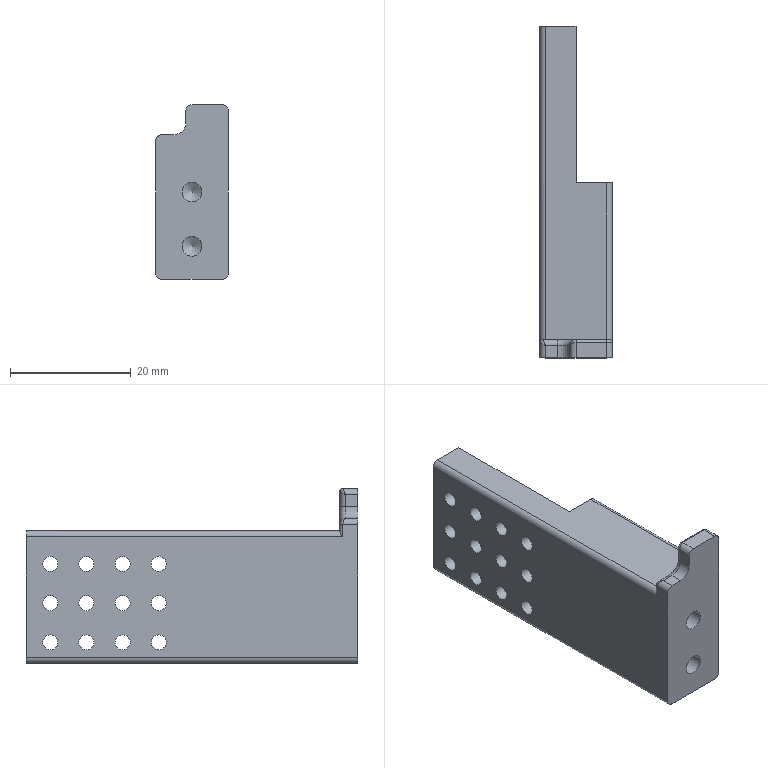CAM job | NX | 3+2 milling, drilling | part box 12 x 55 x 29 mm | stock box 15 x 60 x 34 mm
Tools:
number,name,description,diameter,corner_radius,flute_length,length,flutes
9,D10,平底铣刀-粗,10.0,0.0,35.0,75.0,2
17,D3-J,平底铣刀-精,3.0,0.0,50.0,75.0,2
7,D6-J,平底铣刀-精,6.0,0.0,25.0,75.0,2
10,D10-J,平底铣刀-精,10.0,0.0,35.0,75.0,2
18,D4R0.5,圆鼻刀-粗,4.0,0.5,50.0,75.0,2
1,D80R0.8飞刀,圆鼻刀-粗,80.0,0.8,50.0,75.0,2
2,D6倒角刀,倒角刀,6.0,0.0,3.0,25.0,2
20,M3X0.5,丝锥,2.5,0.0,35.0,50.0,2
12,钻头2.5,Twist Drill 2.5 mm,2.5,0.0,30.0,32.0,2
Operations:
program,operation,operation_type,tool,method,geometry_group,spindle_rpm,surface_speed,feed_per_tooth,feed_cut,feed_plunge,cut_length_mm,path_length_mm,cut_time_min,machine_time_min
B,动态开粗D10_COPY,CavityMilling,D10,动态开粗-切深K-步距K,W-B,8000.0,251.32,0.25,4000.0,100.0,3919.562,3955.362,0.9799,0.9835
B,底壁铣分层开粗-中_COPY,VolumeBased25DMillingOperation,D10,分层开粗-切深K-步距G,W-B,8000.0,251.32,0.25,4000.0,100.0,1576.259,1807.92,0.3941,0.4172
B,等高精光往复爬面_COPY_COPY_1,ZLevelMilling,D4R0.5,等高爬面-切深K-步距G,W-B,7000.0,87.965,0.3214,4500.0,100.0,898.802,925.413,0.1997,0.2024
B,等高精光往复爬面_COPY_COPY_1_COPY,ZLevelMilling,D4R0.5,等高爬面-切深K-步距G,W-B,7000.0,87.965,0.3214,4500.0,100.0,754.856,781.468,0.1677,0.1704
B,平面去毛刺6X45L_COPY,SurfaceContour,D6倒角刀,爬面_倒角-切深0-步距G,W-B,6500.0,122.519,0.1154,1500.0,100.0,132.646,278.125,0.0884,0.103
B,钻倒角_2,Operation,D6倒角刀,METHOD,W-B,7000.0,131.947,0.0357,500.0,0.0,57.0,273.692,0.114,0.1357
B,底壁铣飞面精光_COPY,VolumeBased25DMillingOperation,D10-J,侧刃精光-切深K-步距G,W-B,8000.0,251.32,0.0625,1000.0,100.0,307.415,343.415,0.3074,0.311
B,底壁铣精光底面-中_COPY,VolumeBased25DMillingOperation,D10-J,精光步距切深关,W-B,8000.0,251.32,0.0625,1000.0,100.0,218.805,253.405,0.2188,0.2223
B,底壁铣精光侧面-中-选底面_COPY,VolumeBased25DMillingOperation,D10-J,侧刃精光-切深K-步距G,W-B,8000.0,251.32,0.0625,1000.0,100.0,40.682,76.282,0.0407,0.0442
A,顶面,FaceMilling,D80R0.8飞刀,侧刃精光-切深K-步距G,W-A,5000.0,1256.637,0.1,1000.0,100.0,149.0,185.0,0.149,0.1526
A,型腔铣开粗-中_COPY,CavityMilling,D10,分层开粗-切深K-步距G,W-A,8000.0,251.32,0.25,4000.0,100.0,10835.942,11456.171,2.709,2.802
A,打点-深0.8,Operation,D6倒角刀,NONE,W-A,8000.0,150.796,0.0312,500.0,90.0,21.6,162.098,0.0432,0.0572
A,通孔-M3螺纹底孔,Operation,钻头2.5,NONE,W-A,3000.0,23.562,0.05,300.0,90.0,153.013,424.924,0.51,0.5372
A,外形侧面,ZLevelMilling,D3-J,METHOD,W-A,9000.0,84.823,0.1389,2500.0,80.0,413.7,464.734,0.1656,0.1707
A,等高精光往复爬面_COPY,ZLevelMilling,D4R0.5,等高爬面-切深K-步距G,W-A,7000.0,87.965,0.3214,4500.0,100.0,1378.83,1400.242,0.3064,0.3085
A,等高精光往复爬面_COPY_COPY,ZLevelMilling,D4R0.5,等高爬面-切深K-步距G,W-A,7000.0,87.965,0.3214,4500.0,100.0,1403.019,1424.43,0.3118,0.3139
A,等高精光往复爬面_COPY_COPY_COPY,ZLevelMilling,D4R0.5,等高爬面-切深K-步距G,W-A,7000.0,87.965,0.3214,4500.0,100.0,489.327,514.239,0.1087,0.1112
A,等高精光往复爬面_COPY_COPY_COPY_1,ZLevelMilling,D4R0.5,等高爬面-切深K-步距G,W-A,7000.0,87.965,0.3214,4500.0,100.0,243.79,275.198,0.0542,0.0573
A,仅选体,SurfaceContour,D6倒角刀,METHOD,W-A,8000.0,150.796,0.1875,3000.0,100.0,77.388,274.344,0.0258,0.0455
A,钻倒角_1,Operation,D6倒角刀,METHOD,W-A,8000.0,150.796,0.0312,500.0,0.0,57.0,261.692,0.114,0.1345
A,通孔-攻牙M3,Operation,M3X0.5,METHOD,W-A,800.0,6.283,0.0003,0.5,90.0,120.0,358.898,240.0,240.024
A,等高精光-中_COPY,ZLevelMilling,D6-J,侧刃精光-切深K-步距G,W-A,8000.0,150.792,0.0625,1000.0,100.0,396.71,528.476,0.3967,0.4099